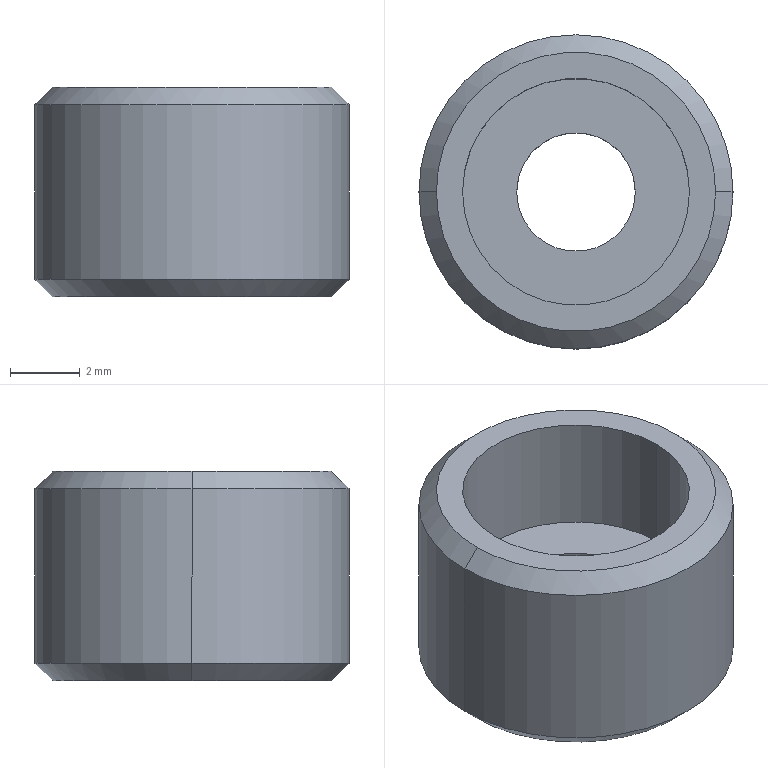Part | STEP file | Anti-rot sleeve | 1 solid | 13 faces | box 9 x 9 x 6 mm | volume 238.468 mm3 | cylinder 6 | cone 4 | plane 3 | commonest cylinder face diameters 3.4 x2 6.5 x2 9 x2
STEP:
#1=CARTESIAN_POINT('',(0.,0.,0.));
#2=DIRECTION('',(0.,0.,1.));
#3=DIRECTION('',(1.,0.,0.));
#4=AXIS2_PLACEMENT_3D('',#1,#2,#3);
#5=CARTESIAN_POINT('',(-4.5,0.,5.5));
#6=VERTEX_POINT('',#5);
#7=CARTESIAN_POINT('',(4.5,0.,5.5));
#8=VERTEX_POINT('',#7);
#9=CARTESIAN_POINT('',(0.,0.,5.5));
#10=DIRECTION('',(0.,0.,-1.));
#11=DIRECTION('',(-1.,0.,0.));
#12=AXIS2_PLACEMENT_3D('',#9,#10,#11);
#13=CIRCLE('',#12,4.5);
#14=CARTESIAN_POINT('',(0.,0.,6.));
#15=DIRECTION('',(0.,0.,-1.));
#16=DIRECTION('',(-1.,0.,0.));
#17=AXIS2_PLACEMENT_3D('',#14,#15,#16);
#18=CYLINDRICAL_SURFACE('',#17,4.5);
#19=CARTESIAN_POINT('',(0.,0.5));
#20=DIRECTION('',(1.,0.));
#21=VECTOR('',#20,1.);
#22=LINE('',#19,#21);
#23=(GEOMETRIC_REPRESENTATION_CONTEXT(2)PARAMETRIC_REPRESENTATION_CONTEXT()REPRESENTATION_CONTEXT('',''));
#24=DEFINITIONAL_REPRESENTATION('',(#22),#23);
#25=PCURVE('',#18,#24);
#26=CARTESIAN_POINT('',(0.,0.,5.5));
#27=DIRECTION('',(0.,0.,-1.));
#28=DIRECTION('',(-1.,0.,0.));
#29=AXIS2_PLACEMENT_3D('',#26,#27,#28);
#30=CONICAL_SURFACE('',#29,4.5,0.7854);
#31=CARTESIAN_POINT('',(0.,0.));
#32=DIRECTION('',(1.,0.));
#33=VECTOR('',#32,1.);
#34=LINE('',#31,#33);
#35=(GEOMETRIC_REPRESENTATION_CONTEXT(2)PARAMETRIC_REPRESENTATION_CONTEXT()REPRESENTATION_CONTEXT('',''));
#36=DEFINITIONAL_REPRESENTATION('',(#34),#35);
#37=PCURVE('',#30,#36);
#38=SURFACE_CURVE('',#13,(#25,#37),.PCURVE_S1.);
#39=EDGE_CURVE('',#6,#8,#38,.T.);
#40=ORIENTED_EDGE('',*,*,#39,.T.);
#41=CARTESIAN_POINT('',(4.5,0.,0.5));
#42=VERTEX_POINT('',#41);
#43=CARTESIAN_POINT('',(4.5,0.,6.));
#44=DIRECTION('',(0.,0.,-1.));
#45=VECTOR('',#44,1.);
#46=LINE('',#43,#45);
#47=CARTESIAN_POINT('',(3.142,0.));
#48=DIRECTION('',(0.,1.));
#49=VECTOR('',#48,1.);
#50=LINE('',#47,#49);
#51=(GEOMETRIC_REPRESENTATION_CONTEXT(2)PARAMETRIC_REPRESENTATION_CONTEXT()REPRESENTATION_CONTEXT('',''));
#52=DEFINITIONAL_REPRESENTATION('',(#50),#51);
#53=PCURVE('',#18,#52);
#54=CARTESIAN_POINT('',(0.,0.,6.));
#55=DIRECTION('',(0.,0.,-1.));
#56=DIRECTION('',(-1.,0.,0.));
#57=AXIS2_PLACEMENT_3D('',#54,#55,#56);
#58=CYLINDRICAL_SURFACE('',#57,4.5);
#59=CARTESIAN_POINT('',(3.142,0.));
#60=DIRECTION('',(0.,1.));
#61=VECTOR('',#60,1.);
#62=LINE('',#59,#61);
#63=(GEOMETRIC_REPRESENTATION_CONTEXT(2)PARAMETRIC_REPRESENTATION_CONTEXT()REPRESENTATION_CONTEXT('',''));
#64=DEFINITIONAL_REPRESENTATION('',(#62),#63);
#65=PCURVE('',#58,#64);
#66=SURFACE_CURVE('',#46,(#53,#65),.PCURVE_S1.);
#67=EDGE_CURVE('',#8,#42,#66,.T.);
#68=ORIENTED_EDGE('',*,*,#67,.T.);
#69=CARTESIAN_POINT('',(-4.5,0.,0.5));
#70=VERTEX_POINT('',#69);
#71=CARTESIAN_POINT('',(0.,0.,0.5));
#72=DIRECTION('',(0.,0.,1.));
#73=DIRECTION('',(-1.,0.,0.));
#74=AXIS2_PLACEMENT_3D('',#71,#72,#73);
#75=CIRCLE('',#74,4.5);
#76=CARTESIAN_POINT('',(6.283,5.5));
#77=DIRECTION('',(-1.,0.));
#78=VECTOR('',#77,1.);
#79=LINE('',#76,#78);
#80=(GEOMETRIC_REPRESENTATION_CONTEXT(2)PARAMETRIC_REPRESENTATION_CONTEXT()REPRESENTATION_CONTEXT('',''));
#81=DEFINITIONAL_REPRESENTATION('',(#79),#80);
#82=PCURVE('',#18,#81);
#83=CARTESIAN_POINT('',(0.,0.,0.5));
#84=DIRECTION('',(0.,0.,1.));
#85=DIRECTION('',(1.,0.,0.));
#86=AXIS2_PLACEMENT_3D('',#83,#84,#85);
#87=CONICAL_SURFACE('',#86,4.5,0.7854);
#88=CARTESIAN_POINT('',(-3.142,0.));
#89=DIRECTION('',(1.,0.));
#90=VECTOR('',#89,1.);
#91=LINE('',#88,#90);
#92=(GEOMETRIC_REPRESENTATION_CONTEXT(2)PARAMETRIC_REPRESENTATION_CONTEXT()REPRESENTATION_CONTEXT('',''));
#93=DEFINITIONAL_REPRESENTATION('',(#91),#92);
#94=PCURVE('',#87,#93);
#95=SURFACE_CURVE('',#75,(#82,#94),.PCURVE_S1.);
#96=EDGE_CURVE('',#42,#70,#95,.T.);
#97=ORIENTED_EDGE('',*,*,#96,.T.);
#98=CARTESIAN_POINT('',(-4.5,0.,6.));
#99=DIRECTION('',(0.,0.,-1.));
#100=VECTOR('',#99,1.);
#101=LINE('',#98,#100);
#102=CARTESIAN_POINT('',(0.,0.));
#103=DIRECTION('',(0.,1.));
#104=VECTOR('',#103,1.);
#105=LINE('',#102,#104);
#106=(GEOMETRIC_REPRESENTATION_CONTEXT(2)PARAMETRIC_REPRESENTATION_CONTEXT()REPRESENTATION_CONTEXT('',''));
#107=DEFINITIONAL_REPRESENTATION('',(#105),#106);
#108=PCURVE('',#18,#107);
#109=CARTESIAN_POINT('',(6.283,0.));
#110=DIRECTION('',(0.,1.));
#111=VECTOR('',#110,1.);
#112=LINE('',#109,#111);
#113=(GEOMETRIC_REPRESENTATION_CONTEXT(2)PARAMETRIC_REPRESENTATION_CONTEXT()REPRESENTATION_CONTEXT('',''));
#114=DEFINITIONAL_REPRESENTATION('',(#112),#113);
#115=PCURVE('',#58,#114);
#116=SURFACE_CURVE('',#101,(#108,#115),.PCURVE_S1.);
#117=EDGE_CURVE('',#6,#70,#116,.T.);
#118=ORIENTED_EDGE('',*,*,#117,.F.);
#119=EDGE_LOOP('',(#40,#68,#97,#118));
#120=FACE_BOUND('',#119,.T.);
#121=ADVANCED_FACE('',(#120),#18,.T.);
#122=CARTESIAN_POINT('',(4.,0.,0.));
#123=VERTEX_POINT('',#122);
#124=CARTESIAN_POINT('',(-4.,0.,0.));
#125=VERTEX_POINT('',#124);
#126=CARTESIAN_POINT('',(0.,0.,0.));
#127=DIRECTION('',(0.,0.,1.));
#128=DIRECTION('',(1.,0.,0.));
#129=AXIS2_PLACEMENT_3D('',#126,#127,#128);
#130=CIRCLE('',#129,4.);
#131=CARTESIAN_POINT('',(0.,-0.5));
#132=DIRECTION('',(1.,0.));
#133=VECTOR('',#132,1.);
#134=LINE('',#131,#133);
#135=(GEOMETRIC_REPRESENTATION_CONTEXT(2)PARAMETRIC_REPRESENTATION_CONTEXT()REPRESENTATION_CONTEXT('',''));
#136=DEFINITIONAL_REPRESENTATION('',(#134),#135);
#137=PCURVE('',#87,#136);
#138=CARTESIAN_POINT('',(0.,0.,0.));
#139=DIRECTION('',(0.,0.,1.));
#140=DIRECTION('',(1.,0.,0.));
#141=AXIS2_PLACEMENT_3D('',#138,#139,#140);
#142=PLANE('',#141);
#143=CARTESIAN_POINT('',(0.,0.));
#144=DIRECTION('',(1.,0.));
#145=AXIS2_PLACEMENT_2D('',#143,#144);
#146=CIRCLE('',#145,4.);
#147=(GEOMETRIC_REPRESENTATION_CONTEXT(2)PARAMETRIC_REPRESENTATION_CONTEXT()REPRESENTATION_CONTEXT('',''));
#148=DEFINITIONAL_REPRESENTATION('',(#146),#147);
#149=PCURVE('',#142,#148);
#150=SURFACE_CURVE('',#130,(#137,#149),.PCURVE_S1.);
#151=EDGE_CURVE('',#123,#125,#150,.T.);
#152=ORIENTED_EDGE('',*,*,#151,.T.);
#153=CARTESIAN_POINT('',(-4.5,0.,0.5));
#154=DIRECTION('',(-0.7071,0.,0.7071));
#155=VECTOR('',#154,1.);
#156=LINE('',#153,#155);
#157=CARTESIAN_POINT('',(3.142,0.));
#158=DIRECTION('',(0.,1.));
#159=VECTOR('',#158,1.);
#160=LINE('',#157,#159);
#161=(GEOMETRIC_REPRESENTATION_CONTEXT(2)PARAMETRIC_REPRESENTATION_CONTEXT()REPRESENTATION_CONTEXT('',''));
#162=DEFINITIONAL_REPRESENTATION('',(#160),#161);
#163=PCURVE('',#87,#162);
#164=CARTESIAN_POINT('',(0.,0.,0.5));
#165=DIRECTION('',(0.,0.,1.));
#166=DIRECTION('',(1.,0.,0.));
#167=AXIS2_PLACEMENT_3D('',#164,#165,#166);
#168=CONICAL_SURFACE('',#167,4.5,0.7854);
#169=CARTESIAN_POINT('',(3.142,0.));
#170=DIRECTION('',(0.,1.));
#171=VECTOR('',#170,1.);
#172=LINE('',#169,#171);
#173=(GEOMETRIC_REPRESENTATION_CONTEXT(2)PARAMETRIC_REPRESENTATION_CONTEXT()REPRESENTATION_CONTEXT('',''));
#174=DEFINITIONAL_REPRESENTATION('',(#172),#173);
#175=PCURVE('',#168,#174);
#176=SURFACE_CURVE('',#156,(#163,#175),.PCURVE_S1.);
#177=EDGE_CURVE('',#125,#70,#176,.T.);
#178=ORIENTED_EDGE('',*,*,#177,.T.);
#179=ORIENTED_EDGE('',*,*,#96,.F.);
#180=CARTESIAN_POINT('',(4.5,0.,0.5));
#181=DIRECTION('',(0.7071,0.,0.7071));
#182=VECTOR('',#181,1.);
#183=LINE('',#180,#182);
#184=CARTESIAN_POINT('',(0.,0.));
#185=DIRECTION('',(0.,1.));
#186=VECTOR('',#185,1.);
#187=LINE('',#184,#186);
#188=(GEOMETRIC_REPRESENTATION_CONTEXT(2)PARAMETRIC_REPRESENTATION_CONTEXT()REPRESENTATION_CONTEXT('',''));
#189=DEFINITIONAL_REPRESENTATION('',(#187),#188);
#190=PCURVE('',#87,#189);
#191=CARTESIAN_POINT('',(6.283,0.));
#192=DIRECTION('',(0.,1.));
#193=VECTOR('',#192,1.);
#194=LINE('',#191,#193);
#195=(GEOMETRIC_REPRESENTATION_CONTEXT(2)PARAMETRIC_REPRESENTATION_CONTEXT()REPRESENTATION_CONTEXT('',''));
#196=DEFINITIONAL_REPRESENTATION('',(#194),#195);
#197=PCURVE('',#168,#196);
#198=SURFACE_CURVE('',#183,(#190,#197),.PCURVE_S1.);
#199=EDGE_CURVE('',#123,#42,#198,.T.);
#200=ORIENTED_EDGE('',*,*,#199,.F.);
#201=EDGE_LOOP('',(#152,#178,#179,#200));
#202=FACE_BOUND('',#201,.T.);
#203=ADVANCED_FACE('',(#202),#87,.T.);
#204=CARTESIAN_POINT('',(-4.,0.,6.));
#205=VERTEX_POINT('',#204);
#206=CARTESIAN_POINT('',(4.,0.,6.));
#207=VERTEX_POINT('',#206);
#208=CARTESIAN_POINT('',(0.,0.,6.));
#209=DIRECTION('',(0.,0.,-1.));
#210=DIRECTION('',(-1.,0.,0.));
#211=AXIS2_PLACEMENT_3D('',#208,#209,#210);
#212=CIRCLE('',#211,4.);
#213=CARTESIAN_POINT('',(0.,-0.5));
#214=DIRECTION('',(1.,0.));
#215=VECTOR('',#214,1.);
#216=LINE('',#213,#215);
#217=(GEOMETRIC_REPRESENTATION_CONTEXT(2)PARAMETRIC_REPRESENTATION_CONTEXT()REPRESENTATION_CONTEXT('',''));
#218=DEFINITIONAL_REPRESENTATION('',(#216),#217);
#219=PCURVE('',#30,#218);
#220=CARTESIAN_POINT('',(0.,0.,6.));
#221=DIRECTION('',(0.,0.,1.));
#222=DIRECTION('',(1.,0.,0.));
#223=AXIS2_PLACEMENT_3D('',#220,#221,#222);
#224=PLANE('',#223);
#225=CARTESIAN_POINT('',(-4.,0.));
#226=CARTESIAN_POINT('',(-4.,6.928));
#227=CARTESIAN_POINT('',(2.,3.464));
#228=CARTESIAN_POINT('',(8.,0.));
#229=CARTESIAN_POINT('',(2.,-3.464));
#230=CARTESIAN_POINT('',(-4.,-6.928));
#231=CARTESIAN_POINT('',(-4.,0.));
#232=(BOUNDED_CURVE()B_SPLINE_CURVE(2,(#225,#226,#227,#228,#229,#230,#231),.UNSPECIFIED.,.T.,.F.)B_SPLINE_CURVE_WITH_KNOTS((1,2,2,2,2,1),(-2.094,0.,2.094,4.189,6.283,8.378),.UNSPECIFIED.)CURVE()GEOMETRIC_REPRESENTATION_ITEM()RATIONAL_B_SPLINE_CURVE((1.,0.5,1.,0.5,1.,0.5,1.))REPRESENTATION_ITEM(''));
#233=(GEOMETRIC_REPRESENTATION_CONTEXT(2)PARAMETRIC_REPRESENTATION_CONTEXT()REPRESENTATION_CONTEXT('',''));
#234=DEFINITIONAL_REPRESENTATION('',(#232),#233);
#235=PCURVE('',#224,#234);
#236=SURFACE_CURVE('',#212,(#219,#235),.PCURVE_S1.);
#237=EDGE_CURVE('',#205,#207,#236,.T.);
#238=ORIENTED_EDGE('',*,*,#237,.T.);
#239=CARTESIAN_POINT('',(4.5,0.,5.5));
#240=DIRECTION('',(0.7071,0.,-0.7071));
#241=VECTOR('',#240,1.);
#242=LINE('',#239,#241);
#243=CARTESIAN_POINT('',(3.142,0.));
#244=DIRECTION('',(0.,1.));
#245=VECTOR('',#244,1.);
#246=LINE('',#243,#245);
#247=(GEOMETRIC_REPRESENTATION_CONTEXT(2)PARAMETRIC_REPRESENTATION_CONTEXT()REPRESENTATION_CONTEXT('',''));
#248=DEFINITIONAL_REPRESENTATION('',(#246),#247);
#249=PCURVE('',#30,#248);
#250=CARTESIAN_POINT('',(0.,0.,5.5));
#251=DIRECTION('',(0.,0.,-1.));
#252=DIRECTION('',(-1.,0.,0.));
#253=AXIS2_PLACEMENT_3D('',#250,#251,#252);
#254=CONICAL_SURFACE('',#253,4.5,0.7854);
#255=CARTESIAN_POINT('',(3.142,0.));
#256=DIRECTION('',(0.,1.));
#257=VECTOR('',#256,1.);
#258=LINE('',#255,#257);
#259=(GEOMETRIC_REPRESENTATION_CONTEXT(2)PARAMETRIC_REPRESENTATION_CONTEXT()REPRESENTATION_CONTEXT('',''));
#260=DEFINITIONAL_REPRESENTATION('',(#258),#259);
#261=PCURVE('',#254,#260);
#262=SURFACE_CURVE('',#242,(#249,#261),.PCURVE_S1.);
#263=EDGE_CURVE('',#207,#8,#262,.T.);
#264=ORIENTED_EDGE('',*,*,#263,.T.);
#265=ORIENTED_EDGE('',*,*,#39,.F.);
#266=CARTESIAN_POINT('',(-4.5,0.,5.5));
#267=DIRECTION('',(-0.7071,0.,-0.7071));
#268=VECTOR('',#267,1.);
#269=LINE('',#266,#268);
#270=CARTESIAN_POINT('',(0.,0.));
#271=DIRECTION('',(0.,1.));
#272=VECTOR('',#271,1.);
#273=LINE('',#270,#272);
#274=(GEOMETRIC_REPRESENTATION_CONTEXT(2)PARAMETRIC_REPRESENTATION_CONTEXT()REPRESENTATION_CONTEXT('',''));
#275=DEFINITIONAL_REPRESENTATION('',(#273),#274);
#276=PCURVE('',#30,#275);
#277=CARTESIAN_POINT('',(6.283,0.));
#278=DIRECTION('',(0.,1.));
#279=VECTOR('',#278,1.);
#280=LINE('',#277,#279);
#281=(GEOMETRIC_REPRESENTATION_CONTEXT(2)PARAMETRIC_REPRESENTATION_CONTEXT()REPRESENTATION_CONTEXT('',''));
#282=DEFINITIONAL_REPRESENTATION('',(#280),#281);
#283=PCURVE('',#254,#282);
#284=SURFACE_CURVE('',#269,(#276,#283),.PCURVE_S1.);
#285=EDGE_CURVE('',#205,#6,#284,.T.);
#286=ORIENTED_EDGE('',*,*,#285,.F.);
#287=EDGE_LOOP('',(#238,#264,#265,#286));
#288=FACE_BOUND('',#287,.T.);
#289=ADVANCED_FACE('',(#288),#30,.T.);
#290=CARTESIAN_POINT('',(1.7,0.,0.));
#291=VERTEX_POINT('',#290);
#292=CARTESIAN_POINT('',(1.7,0.,2.6));
#293=VERTEX_POINT('',#292);
#294=CARTESIAN_POINT('',(1.7,0.,6.));
#295=DIRECTION('',(0.,0.,1.));
#296=VECTOR('',#295,1.);
#297=LINE('',#294,#296);
#298=CARTESIAN_POINT('',(0.,0.,6.));
#299=DIRECTION('',(0.,0.,1.));
#300=DIRECTION('',(1.,0.,0.));
#301=AXIS2_PLACEMENT_3D('',#298,#299,#300);
#302=CYLINDRICAL_SURFACE('',#301,1.7);
#303=CARTESIAN_POINT('',(6.283,0.));
#304=DIRECTION('',(0.,1.));
#305=VECTOR('',#304,1.);
#306=LINE('',#303,#305);
#307=(GEOMETRIC_REPRESENTATION_CONTEXT(2)PARAMETRIC_REPRESENTATION_CONTEXT()REPRESENTATION_CONTEXT('',''));
#308=DEFINITIONAL_REPRESENTATION('',(#306),#307);
#309=PCURVE('',#302,#308);
#310=CARTESIAN_POINT('',(0.,0.,6.));
#311=DIRECTION('',(0.,0.,1.));
#312=DIRECTION('',(1.,0.,0.));
#313=AXIS2_PLACEMENT_3D('',#310,#311,#312);
#314=CYLINDRICAL_SURFACE('',#313,1.7);
#315=CARTESIAN_POINT('',(0.,0.));
#316=DIRECTION('',(0.,1.));
#317=VECTOR('',#316,1.);
#318=LINE('',#315,#317);
#319=(GEOMETRIC_REPRESENTATION_CONTEXT(2)PARAMETRIC_REPRESENTATION_CONTEXT()REPRESENTATION_CONTEXT('',''));
#320=DEFINITIONAL_REPRESENTATION('',(#318),#319);
#321=PCURVE('',#314,#320);
#322=SURFACE_CURVE('',#297,(#309,#321),.PCURVE_S1.);
#323=EDGE_CURVE('',#291,#293,#322,.T.);
#324=ORIENTED_EDGE('',*,*,#323,.T.);
#325=CARTESIAN_POINT('',(-1.7,0.,2.6));
#326=VERTEX_POINT('',#325);
#327=CARTESIAN_POINT('',(0.,0.,2.6));
#328=DIRECTION('',(0.,0.,-1.));
#329=DIRECTION('',(1.,0.,0.));
#330=AXIS2_PLACEMENT_3D('',#327,#328,#329);
#331=CIRCLE('',#330,1.7);
#332=CARTESIAN_POINT('',(6.283,-3.4));
#333=DIRECTION('',(-1.,0.));
#334=VECTOR('',#333,1.);
#335=LINE('',#332,#334);
#336=(GEOMETRIC_REPRESENTATION_CONTEXT(2)PARAMETRIC_REPRESENTATION_CONTEXT()REPRESENTATION_CONTEXT('',''));
#337=DEFINITIONAL_REPRESENTATION('',(#335),#336);
#338=PCURVE('',#302,#337);
#339=CARTESIAN_POINT('',(1.7,0.,2.6));
#340=DIRECTION('',(0.,0.,-1.));
#341=DIRECTION('',(-1.,0.,0.));
#342=AXIS2_PLACEMENT_3D('',#339,#340,#341);
#343=PLANE('',#342);
#344=CARTESIAN_POINT('',(1.7,0.));
#345=DIRECTION('',(-1.,0.));
#346=AXIS2_PLACEMENT_2D('',#344,#345);
#347=CIRCLE('',#346,1.7);
#348=(GEOMETRIC_REPRESENTATION_CONTEXT(2)PARAMETRIC_REPRESENTATION_CONTEXT()REPRESENTATION_CONTEXT('',''));
#349=DEFINITIONAL_REPRESENTATION('',(#347),#348);
#350=PCURVE('',#343,#349);
#351=SURFACE_CURVE('',#331,(#338,#350),.PCURVE_S1.);
#352=EDGE_CURVE('',#293,#326,#351,.T.);
#353=ORIENTED_EDGE('',*,*,#352,.T.);
#354=CARTESIAN_POINT('',(-1.7,0.,0.));
#355=VERTEX_POINT('',#354);
#356=CARTESIAN_POINT('',(-1.7,0.,6.));
#357=DIRECTION('',(0.,0.,1.));
#358=VECTOR('',#357,1.);
#359=LINE('',#356,#358);
#360=CARTESIAN_POINT('',(3.142,0.));
#361=DIRECTION('',(0.,1.));
#362=VECTOR('',#361,1.);
#363=LINE('',#360,#362);
#364=(GEOMETRIC_REPRESENTATION_CONTEXT(2)PARAMETRIC_REPRESENTATION_CONTEXT()REPRESENTATION_CONTEXT('',''));
#365=DEFINITIONAL_REPRESENTATION('',(#363),#364);
#366=PCURVE('',#302,#365);
#367=CARTESIAN_POINT('',(3.142,0.));
#368=DIRECTION('',(0.,1.));
#369=VECTOR('',#368,1.);
#370=LINE('',#367,#369);
#371=(GEOMETRIC_REPRESENTATION_CONTEXT(2)PARAMETRIC_REPRESENTATION_CONTEXT()REPRESENTATION_CONTEXT('',''));
#372=DEFINITIONAL_REPRESENTATION('',(#370),#371);
#373=PCURVE('',#314,#372);
#374=SURFACE_CURVE('',#359,(#366,#373),.PCURVE_S1.);
#375=EDGE_CURVE('',#355,#326,#374,.T.);
#376=ORIENTED_EDGE('',*,*,#375,.F.);
#377=CARTESIAN_POINT('',(0.,0.,0.));
#378=DIRECTION('',(0.,0.,-1.));
#379=DIRECTION('',(1.,0.,0.));
#380=AXIS2_PLACEMENT_3D('',#377,#378,#379);
#381=CIRCLE('',#380,1.7);
#382=CARTESIAN_POINT('',(6.283,-6.));
#383=DIRECTION('',(-1.,0.));
#384=VECTOR('',#383,1.);
#385=LINE('',#382,#384);
#386=(GEOMETRIC_REPRESENTATION_CONTEXT(2)PARAMETRIC_REPRESENTATION_CONTEXT()REPRESENTATION_CONTEXT('',''));
#387=DEFINITIONAL_REPRESENTATION('',(#385),#386);
#388=PCURVE('',#302,#387);
#389=CARTESIAN_POINT('',(1.7,0.));
#390=CARTESIAN_POINT('',(1.7,-2.944));
#391=CARTESIAN_POINT('',(-0.85,-1.472));
#392=CARTESIAN_POINT('',(-3.4,0.));
#393=CARTESIAN_POINT('',(-0.85,1.472));
#394=CARTESIAN_POINT('',(1.7,2.944));
#395=CARTESIAN_POINT('',(1.7,0.));
#396=(BOUNDED_CURVE()B_SPLINE_CURVE(2,(#389,#390,#391,#392,#393,#394,#395),.UNSPECIFIED.,.T.,.F.)B_SPLINE_CURVE_WITH_KNOTS((1,2,2,2,2,1),(-2.094,0.,2.094,4.189,6.283,8.378),.UNSPECIFIED.)CURVE()GEOMETRIC_REPRESENTATION_ITEM()RATIONAL_B_SPLINE_CURVE((1.,0.5,1.,0.5,1.,0.5,1.))REPRESENTATION_ITEM(''));
#397=(GEOMETRIC_REPRESENTATION_CONTEXT(2)PARAMETRIC_REPRESENTATION_CONTEXT()REPRESENTATION_CONTEXT('',''));
#398=DEFINITIONAL_REPRESENTATION('',(#396),#397);
#399=PCURVE('',#142,#398);
#400=SURFACE_CURVE('',#381,(#388,#399),.PCURVE_S1.);
#401=EDGE_CURVE('',#291,#355,#400,.T.);
#402=ORIENTED_EDGE('',*,*,#401,.F.);
#403=EDGE_LOOP('',(#324,#353,#376,#402));
#404=FACE_BOUND('',#403,.F.);
#405=ADVANCED_FACE('',(#404),#302,.F.);
#406=CARTESIAN_POINT('',(3.25,0.,2.6));
#407=VERTEX_POINT('',#406);
#408=CARTESIAN_POINT('',(3.25,0.,6.));
#409=VERTEX_POINT('',#408);
#410=CARTESIAN_POINT('',(3.25,0.,6.));
#411=DIRECTION('',(0.,0.,1.));
#412=VECTOR('',#411,1.);
#413=LINE('',#410,#412);
#414=CARTESIAN_POINT('',(0.,0.,6.));
#415=DIRECTION('',(0.,0.,1.));
#416=DIRECTION('',(1.,0.,0.));
#417=AXIS2_PLACEMENT_3D('',#414,#415,#416);
#418=CYLINDRICAL_SURFACE('',#417,3.25);
#419=CARTESIAN_POINT('',(6.283,0.));
#420=DIRECTION('',(0.,1.));
#421=VECTOR('',#420,1.);
#422=LINE('',#419,#421);
#423=(GEOMETRIC_REPRESENTATION_CONTEXT(2)PARAMETRIC_REPRESENTATION_CONTEXT()REPRESENTATION_CONTEXT('',''));
#424=DEFINITIONAL_REPRESENTATION('',(#422),#423);
#425=PCURVE('',#418,#424);
#426=CARTESIAN_POINT('',(0.,0.,6.));
#427=DIRECTION('',(0.,0.,1.));
#428=DIRECTION('',(1.,0.,0.));
#429=AXIS2_PLACEMENT_3D('',#426,#427,#428);
#430=CYLINDRICAL_SURFACE('',#429,3.25);
#431=CARTESIAN_POINT('',(0.,0.));
#432=DIRECTION('',(0.,1.));
#433=VECTOR('',#432,1.);
#434=LINE('',#431,#433);
#435=(GEOMETRIC_REPRESENTATION_CONTEXT(2)PARAMETRIC_REPRESENTATION_CONTEXT()REPRESENTATION_CONTEXT('',''));
#436=DEFINITIONAL_REPRESENTATION('',(#434),#435);
#437=PCURVE('',#430,#436);
#438=SURFACE_CURVE('',#413,(#425,#437),.PCURVE_S1.);
#439=EDGE_CURVE('',#407,#409,#438,.T.);
#440=ORIENTED_EDGE('',*,*,#439,.T.);
#441=CARTESIAN_POINT('',(-3.25,0.,6.));
#442=VERTEX_POINT('',#441);
#443=CARTESIAN_POINT('',(0.,0.,6.));
#444=DIRECTION('',(0.,0.,-1.));
#445=DIRECTION('',(1.,0.,0.));
#446=AXIS2_PLACEMENT_3D('',#443,#444,#445);
#447=CIRCLE('',#446,3.25);
#448=CARTESIAN_POINT('',(6.283,0.));
#449=DIRECTION('',(-1.,0.));
#450=VECTOR('',#449,1.);
#451=LINE('',#448,#450);
#452=(GEOMETRIC_REPRESENTATION_CONTEXT(2)PARAMETRIC_REPRESENTATION_CONTEXT()REPRESENTATION_CONTEXT('',''));
#453=DEFINITIONAL_REPRESENTATION('',(#451),#452);
#454=PCURVE('',#418,#453);
#455=CARTESIAN_POINT('',(3.25,0.));
#456=CARTESIAN_POINT('',(3.25,-5.629));
#457=CARTESIAN_POINT('',(-1.625,-2.815));
#458=CARTESIAN_POINT('',(-6.5,0.));
#459=CARTESIAN_POINT('',(-1.625,2.815));
#460=CARTESIAN_POINT('',(3.25,5.629));
#461=CARTESIAN_POINT('',(3.25,0.));
#462=(BOUNDED_CURVE()B_SPLINE_CURVE(2,(#455,#456,#457,#458,#459,#460,#461),.UNSPECIFIED.,.T.,.F.)B_SPLINE_CURVE_WITH_KNOTS((1,2,2,2,2,1),(-2.094,0.,2.094,4.189,6.283,8.378),.UNSPECIFIED.)CURVE()GEOMETRIC_REPRESENTATION_ITEM()RATIONAL_B_SPLINE_CURVE((1.,0.5,1.,0.5,1.,0.5,1.))REPRESENTATION_ITEM(''));
#463=(GEOMETRIC_REPRESENTATION_CONTEXT(2)PARAMETRIC_REPRESENTATION_CONTEXT()REPRESENTATION_CONTEXT('',''));
#464=DEFINITIONAL_REPRESENTATION('',(#462),#463);
#465=PCURVE('',#224,#464);
#466=SURFACE_CURVE('',#447,(#454,#465),.PCURVE_S1.);
#467=EDGE_CURVE('',#409,#442,#466,.T.);
#468=ORIENTED_EDGE('',*,*,#467,.T.);
#469=CARTESIAN_POINT('',(-3.25,0.,2.6));
#470=VERTEX_POINT('',#469);
#471=CARTESIAN_POINT('',(-3.25,0.,6.));
#472=DIRECTION('',(0.,0.,1.));
#473=VECTOR('',#472,1.);
#474=LINE('',#471,#473);
#475=CARTESIAN_POINT('',(3.142,0.));
#476=DIRECTION('',(0.,1.));
#477=VECTOR('',#476,1.);
#478=LINE('',#475,#477);
#479=(GEOMETRIC_REPRESENTATION_CONTEXT(2)PARAMETRIC_REPRESENTATION_CONTEXT()REPRESENTATION_CONTEXT('',''));
#480=DEFINITIONAL_REPRESENTATION('',(#478),#479);
#481=PCURVE('',#418,#480);
#482=CARTESIAN_POINT('',(3.142,0.));
#483=DIRECTION('',(0.,1.));
#484=VECTOR('',#483,1.);
#485=LINE('',#482,#484);
#486=(GEOMETRIC_REPRESENTATION_CONTEXT(2)PARAMETRIC_REPRESENTATION_CONTEXT()REPRESENTATION_CONTEXT('',''));
#487=DEFINITIONAL_REPRESENTATION('',(#485),#486);
#488=PCURVE('',#430,#487);
#489=SURFACE_CURVE('',#474,(#481,#488),.PCURVE_S1.);
#490=EDGE_CURVE('',#470,#442,#489,.T.);
#491=ORIENTED_EDGE('',*,*,#490,.F.);
#492=CARTESIAN_POINT('',(0.,0.,2.6));
#493=DIRECTION('',(0.,0.,1.));
#494=DIRECTION('',(1.,0.,0.));
#495=AXIS2_PLACEMENT_3D('',#492,#493,#494);
#496=CIRCLE('',#495,3.25);
#497=CARTESIAN_POINT('',(0.,-3.4));
#498=DIRECTION('',(1.,0.));
#499=VECTOR('',#498,1.);
#500=LINE('',#497,#499);
#501=(GEOMETRIC_REPRESENTATION_CONTEXT(2)PARAMETRIC_REPRESENTATION_CONTEXT()REPRESENTATION_CONTEXT('',''));
#502=DEFINITIONAL_REPRESENTATION('',(#500),#501);
#503=PCURVE('',#418,#502);
#504=CARTESIAN_POINT('',(-1.55,0.));
#505=CARTESIAN_POINT('',(-1.55,5.629));
#506=CARTESIAN_POINT('',(3.325,2.815));
#507=CARTESIAN_POINT('',(8.2,0.));
#508=CARTESIAN_POINT('',(3.325,-2.815));
#509=CARTESIAN_POINT('',(-1.55,-5.629));
#510=CARTESIAN_POINT('',(-1.55,0.));
#511=(BOUNDED_CURVE()B_SPLINE_CURVE(2,(#504,#505,#506,#507,#508,#509,#510),.UNSPECIFIED.,.T.,.F.)B_SPLINE_CURVE_WITH_KNOTS((1,2,2,2,2,1),(-2.094,0.,2.094,4.189,6.283,8.378),.UNSPECIFIED.)CURVE()GEOMETRIC_REPRESENTATION_ITEM()RATIONAL_B_SPLINE_CURVE((1.,0.5,1.,0.5,1.,0.5,1.))REPRESENTATION_ITEM(''));
#512=(GEOMETRIC_REPRESENTATION_CONTEXT(2)PARAMETRIC_REPRESENTATION_CONTEXT()REPRESENTATION_CONTEXT('',''));
#513=DEFINITIONAL_REPRESENTATION('',(#511),#512);
#514=PCURVE('',#343,#513);
#515=SURFACE_CURVE('',#496,(#503,#514),.PCURVE_S1.);
#516=EDGE_CURVE('',#470,#407,#515,.T.);
#517=ORIENTED_EDGE('',*,*,#516,.T.);
#518=EDGE_LOOP('',(#440,#468,#491,#517));
#519=FACE_BOUND('',#518,.F.);
#520=ADVANCED_FACE('',(#519),#418,.F.);
#521=ORIENTED_EDGE('',*,*,#67,.F.);
#522=CARTESIAN_POINT('',(0.,0.,5.5));
#523=DIRECTION('',(0.,0.,-1.));
#524=DIRECTION('',(-1.,0.,0.));
#525=AXIS2_PLACEMENT_3D('',#522,#523,#524);
#526=CIRCLE('',#525,4.5);
#527=CARTESIAN_POINT('',(0.,0.5));
#528=DIRECTION('',(1.,0.));
#529=VECTOR('',#528,1.);
#530=LINE('',#527,#529);
#531=(GEOMETRIC_REPRESENTATION_CONTEXT(2)PARAMETRIC_REPRESENTATION_CONTEXT()REPRESENTATION_CONTEXT('',''));
#532=DEFINITIONAL_REPRESENTATION('',(#530),#531);
#533=PCURVE('',#58,#532);
#534=CARTESIAN_POINT('',(0.,0.));
#535=DIRECTION('',(1.,0.));
#536=VECTOR('',#535,1.);
#537=LINE('',#534,#536);
#538=(GEOMETRIC_REPRESENTATION_CONTEXT(2)PARAMETRIC_REPRESENTATION_CONTEXT()REPRESENTATION_CONTEXT('',''));
#539=DEFINITIONAL_REPRESENTATION('',(#537),#538);
#540=PCURVE('',#254,#539);
#541=SURFACE_CURVE('',#526,(#533,#540),.PCURVE_S1.);
#542=EDGE_CURVE('',#8,#6,#541,.T.);
#543=ORIENTED_EDGE('',*,*,#542,.T.);
#544=ORIENTED_EDGE('',*,*,#117,.T.);
#545=CARTESIAN_POINT('',(0.,0.,0.5));
#546=DIRECTION('',(0.,0.,1.));
#547=DIRECTION('',(-1.,0.,0.));
#548=AXIS2_PLACEMENT_3D('',#545,#546,#547);
#549=CIRCLE('',#548,4.5);
#550=CARTESIAN_POINT('',(6.283,5.5));
#551=DIRECTION('',(-1.,0.));
#552=VECTOR('',#551,1.);
#553=LINE('',#550,#552);
#554=(GEOMETRIC_REPRESENTATION_CONTEXT(2)PARAMETRIC_REPRESENTATION_CONTEXT()REPRESENTATION_CONTEXT('',''));
#555=DEFINITIONAL_REPRESENTATION('',(#553),#554);
#556=PCURVE('',#58,#555);
#557=CARTESIAN_POINT('',(3.142,0.));
#558=DIRECTION('',(1.,0.));
#559=VECTOR('',#558,1.);
#560=LINE('',#557,#559);
#561=(GEOMETRIC_REPRESENTATION_CONTEXT(2)PARAMETRIC_REPRESENTATION_CONTEXT()REPRESENTATION_CONTEXT('',''));
#562=DEFINITIONAL_REPRESENTATION('',(#560),#561);
#563=PCURVE('',#168,#562);
#564=SURFACE_CURVE('',#549,(#556,#563),.PCURVE_S1.);
#565=EDGE_CURVE('',#70,#42,#564,.T.);
#566=ORIENTED_EDGE('',*,*,#565,.T.);
#567=EDGE_LOOP('',(#521,#543,#544,#566));
#568=FACE_BOUND('',#567,.T.);
#569=ADVANCED_FACE('',(#568),#58,.T.);
#570=ORIENTED_EDGE('',*,*,#177,.F.);
#571=CARTESIAN_POINT('',(0.,0.,0.));
#572=DIRECTION('',(0.,0.,1.));
#573=DIRECTION('',(1.,0.,0.));
#574=AXIS2_PLACEMENT_3D('',#571,#572,#573);
#575=CIRCLE('',#574,4.);
#576=CARTESIAN_POINT('',(0.,-0.5));
#577=DIRECTION('',(1.,0.));
#578=VECTOR('',#577,1.);
#579=LINE('',#576,#578);
#580=(GEOMETRIC_REPRESENTATION_CONTEXT(2)PARAMETRIC_REPRESENTATION_CONTEXT()REPRESENTATION_CONTEXT('',''));
#581=DEFINITIONAL_REPRESENTATION('',(#579),#580);
#582=PCURVE('',#168,#581);
#583=CARTESIAN_POINT('',(0.,0.));
#584=DIRECTION('',(1.,0.));
#585=AXIS2_PLACEMENT_2D('',#583,#584);
#586=CIRCLE('',#585,4.);
#587=(GEOMETRIC_REPRESENTATION_CONTEXT(2)PARAMETRIC_REPRESENTATION_CONTEXT()REPRESENTATION_CONTEXT('',''));
#588=DEFINITIONAL_REPRESENTATION('',(#586),#587);
#589=PCURVE('',#142,#588);
#590=SURFACE_CURVE('',#575,(#582,#589),.PCURVE_S1.);
#591=EDGE_CURVE('',#125,#123,#590,.T.);
#592=ORIENTED_EDGE('',*,*,#591,.T.);
#593=ORIENTED_EDGE('',*,*,#199,.T.);
#594=ORIENTED_EDGE('',*,*,#565,.F.);
#595=EDGE_LOOP('',(#570,#592,#593,#594));
#596=FACE_BOUND('',#595,.T.);
#597=ADVANCED_FACE('',(#596),#168,.T.);
#598=ORIENTED_EDGE('',*,*,#263,.F.);
#599=CARTESIAN_POINT('',(0.,0.,6.));
#600=DIRECTION('',(0.,0.,-1.));
#601=DIRECTION('',(-1.,0.,0.));
#602=AXIS2_PLACEMENT_3D('',#599,#600,#601);
#603=CIRCLE('',#602,4.);
#604=CARTESIAN_POINT('',(0.,-0.5));
#605=DIRECTION('',(1.,0.));
#606=VECTOR('',#605,1.);
#607=LINE('',#604,#606);
#608=(GEOMETRIC_REPRESENTATION_CONTEXT(2)PARAMETRIC_REPRESENTATION_CONTEXT()REPRESENTATION_CONTEXT('',''));
#609=DEFINITIONAL_REPRESENTATION('',(#607),#608);
#610=PCURVE('',#254,#609);
#611=CARTESIAN_POINT('',(-4.,0.));
#612=CARTESIAN_POINT('',(-4.,6.928));
#613=CARTESIAN_POINT('',(2.,3.464));
#614=CARTESIAN_POINT('',(8.,0.));
#615=CARTESIAN_POINT('',(2.,-3.464));
#616=CARTESIAN_POINT('',(-4.,-6.928));
#617=CARTESIAN_POINT('',(-4.,0.));
#618=(BOUNDED_CURVE()B_SPLINE_CURVE(2,(#611,#612,#613,#614,#615,#616,#617),.UNSPECIFIED.,.T.,.F.)B_SPLINE_CURVE_WITH_KNOTS((1,2,2,2,2,1),(-2.094,0.,2.094,4.189,6.283,8.378),.UNSPECIFIED.)CURVE()GEOMETRIC_REPRESENTATION_ITEM()RATIONAL_B_SPLINE_CURVE((1.,0.5,1.,0.5,1.,0.5,1.))REPRESENTATION_ITEM(''));
#619=(GEOMETRIC_REPRESENTATION_CONTEXT(2)PARAMETRIC_REPRESENTATION_CONTEXT()REPRESENTATION_CONTEXT('',''));
#620=DEFINITIONAL_REPRESENTATION('',(#618),#619);
#621=PCURVE('',#224,#620);
#622=SURFACE_CURVE('',#603,(#610,#621),.PCURVE_S1.);
#623=EDGE_CURVE('',#207,#205,#622,.T.);
#624=ORIENTED_EDGE('',*,*,#623,.T.);
#625=ORIENTED_EDGE('',*,*,#285,.T.);
#626=ORIENTED_EDGE('',*,*,#542,.F.);
#627=EDGE_LOOP('',(#598,#624,#625,#626));
#628=FACE_BOUND('',#627,.T.);
#629=ADVANCED_FACE('',(#628),#254,.T.);
#630=ORIENTED_EDGE('',*,*,#401,.F.);
#631=CARTESIAN_POINT('',(0.,0.,0.));
#632=DIRECTION('',(0.,0.,-1.));
#633=DIRECTION('',(1.,0.,0.));
#634=AXIS2_PLACEMENT_3D('',#631,#632,#633);
#635=CIRCLE('',#634,1.7);
#636=CARTESIAN_POINT('',(1.7,0.));
#637=CARTESIAN_POINT('',(1.7,-2.944));
#638=CARTESIAN_POINT('',(-0.85,-1.472));
#639=CARTESIAN_POINT('',(-3.4,0.));
#640=CARTESIAN_POINT('',(-0.85,1.472));
#641=CARTESIAN_POINT('',(1.7,2.944));
#642=CARTESIAN_POINT('',(1.7,0.));
#643=(BOUNDED_CURVE()B_SPLINE_CURVE(2,(#636,#637,#638,#639,#640,#641,#642),.UNSPECIFIED.,.T.,.F.)B_SPLINE_CURVE_WITH_KNOTS((1,2,2,2,2,1),(-2.094,0.,2.094,4.189,6.283,8.378),.UNSPECIFIED.)CURVE()GEOMETRIC_REPRESENTATION_ITEM()RATIONAL_B_SPLINE_CURVE((1.,0.5,1.,0.5,1.,0.5,1.))REPRESENTATION_ITEM(''));
#644=(GEOMETRIC_REPRESENTATION_CONTEXT(2)PARAMETRIC_REPRESENTATION_CONTEXT()REPRESENTATION_CONTEXT('',''));
#645=DEFINITIONAL_REPRESENTATION('',(#643),#644);
#646=PCURVE('',#142,#645);
#647=CARTESIAN_POINT('',(6.283,-6.));
#648=DIRECTION('',(-1.,0.));
#649=VECTOR('',#648,1.);
#650=LINE('',#647,#649);
#651=(GEOMETRIC_REPRESENTATION_CONTEXT(2)PARAMETRIC_REPRESENTATION_CONTEXT()REPRESENTATION_CONTEXT('',''));
#652=DEFINITIONAL_REPRESENTATION('',(#650),#651);
#653=PCURVE('',#314,#652);
#654=SURFACE_CURVE('',#635,(#646,#653),.PCURVE_S1.);
#655=EDGE_CURVE('',#355,#291,#654,.T.);
#656=ORIENTED_EDGE('',*,*,#655,.F.);
#657=EDGE_LOOP('',(#630,#656));
#658=FACE_BOUND('',#657,.T.);
#659=ORIENTED_EDGE('',*,*,#151,.F.);
#660=ORIENTED_EDGE('',*,*,#591,.F.);
#661=EDGE_LOOP('',(#659,#660));
#662=FACE_BOUND('',#661,.T.);
#663=ADVANCED_FACE('',(#658,#662),#142,.F.);
#664=ORIENTED_EDGE('',*,*,#467,.T.);
#665=CARTESIAN_POINT('',(0.,0.,6.));
#666=DIRECTION('',(0.,0.,-1.));
#667=DIRECTION('',(1.,0.,0.));
#668=AXIS2_PLACEMENT_3D('',#665,#666,#667);
#669=CIRCLE('',#668,3.25);
#670=CARTESIAN_POINT('',(3.25,0.));
#671=CARTESIAN_POINT('',(3.25,-5.629));
#672=CARTESIAN_POINT('',(-1.625,-2.815));
#673=CARTESIAN_POINT('',(-6.5,0.));
#674=CARTESIAN_POINT('',(-1.625,2.815));
#675=CARTESIAN_POINT('',(3.25,5.629));
#676=CARTESIAN_POINT('',(3.25,0.));
#677=(BOUNDED_CURVE()B_SPLINE_CURVE(2,(#670,#671,#672,#673,#674,#675,#676),.UNSPECIFIED.,.T.,.F.)B_SPLINE_CURVE_WITH_KNOTS((1,2,2,2,2,1),(-2.094,0.,2.094,4.189,6.283,8.378),.UNSPECIFIED.)CURVE()GEOMETRIC_REPRESENTATION_ITEM()RATIONAL_B_SPLINE_CURVE((1.,0.5,1.,0.5,1.,0.5,1.))REPRESENTATION_ITEM(''));
#678=(GEOMETRIC_REPRESENTATION_CONTEXT(2)PARAMETRIC_REPRESENTATION_CONTEXT()REPRESENTATION_CONTEXT('',''));
#679=DEFINITIONAL_REPRESENTATION('',(#677),#678);
#680=PCURVE('',#224,#679);
#681=CARTESIAN_POINT('',(6.283,0.));
#682=DIRECTION('',(-1.,0.));
#683=VECTOR('',#682,1.);
#684=LINE('',#681,#683);
#685=(GEOMETRIC_REPRESENTATION_CONTEXT(2)PARAMETRIC_REPRESENTATION_CONTEXT()REPRESENTATION_CONTEXT('',''));
#686=DEFINITIONAL_REPRESENTATION('',(#684),#685);
#687=PCURVE('',#430,#686);
#688=SURFACE_CURVE('',#669,(#680,#687),.PCURVE_S1.);
#689=EDGE_CURVE('',#442,#409,#688,.T.);
#690=ORIENTED_EDGE('',*,*,#689,.T.);
#691=EDGE_LOOP('',(#664,#690));
#692=FACE_BOUND('',#691,.T.);
#693=ORIENTED_EDGE('',*,*,#237,.F.);
#694=ORIENTED_EDGE('',*,*,#623,.F.);
#695=EDGE_LOOP('',(#693,#694));
#696=FACE_BOUND('',#695,.T.);
#697=ADVANCED_FACE('',(#692,#696),#224,.T.);
#698=CARTESIAN_POINT('',(0.,0.,2.6));
#699=DIRECTION('',(0.,0.,-1.));
#700=DIRECTION('',(1.,0.,0.));
#701=AXIS2_PLACEMENT_3D('',#698,#699,#700);
#702=CIRCLE('',#701,1.7);
#703=CARTESIAN_POINT('',(6.283,-3.4));
#704=DIRECTION('',(-1.,0.));
#705=VECTOR('',#704,1.);
#706=LINE('',#703,#705);
#707=(GEOMETRIC_REPRESENTATION_CONTEXT(2)PARAMETRIC_REPRESENTATION_CONTEXT()REPRESENTATION_CONTEXT('',''));
#708=DEFINITIONAL_REPRESENTATION('',(#706),#707);
#709=PCURVE('',#314,#708);
#710=CARTESIAN_POINT('',(1.7,0.));
#711=DIRECTION('',(-1.,0.));
#712=AXIS2_PLACEMENT_2D('',#710,#711);
#713=CIRCLE('',#712,1.7);
#714=(GEOMETRIC_REPRESENTATION_CONTEXT(2)PARAMETRIC_REPRESENTATION_CONTEXT()REPRESENTATION_CONTEXT('',''));
#715=DEFINITIONAL_REPRESENTATION('',(#713),#714);
#716=PCURVE('',#343,#715);
#717=SURFACE_CURVE('',#702,(#709,#716),.PCURVE_S1.);
#718=EDGE_CURVE('',#326,#293,#717,.T.);
#719=ORIENTED_EDGE('',*,*,#718,.T.);
#720=ORIENTED_EDGE('',*,*,#323,.F.);
#721=ORIENTED_EDGE('',*,*,#655,.F.);
#722=ORIENTED_EDGE('',*,*,#375,.T.);
#723=EDGE_LOOP('',(#719,#720,#721,#722));
#724=FACE_BOUND('',#723,.F.);
#725=ADVANCED_FACE('',(#724),#314,.F.);
#726=ORIENTED_EDGE('',*,*,#689,.T.);
#727=ORIENTED_EDGE('',*,*,#439,.F.);
#728=CARTESIAN_POINT('',(0.,0.,2.6));
#729=DIRECTION('',(0.,0.,1.));
#730=DIRECTION('',(1.,0.,0.));
#731=AXIS2_PLACEMENT_3D('',#728,#729,#730);
#732=CIRCLE('',#731,3.25);
#733=CARTESIAN_POINT('',(0.,-3.4));
#734=DIRECTION('',(1.,0.));
#735=VECTOR('',#734,1.);
#736=LINE('',#733,#735);
#737=(GEOMETRIC_REPRESENTATION_CONTEXT(2)PARAMETRIC_REPRESENTATION_CONTEXT()REPRESENTATION_CONTEXT('',''));
#738=DEFINITIONAL_REPRESENTATION('',(#736),#737);
#739=PCURVE('',#430,#738);
#740=CARTESIAN_POINT('',(-1.55,0.));
#741=CARTESIAN_POINT('',(-1.55,5.629));
#742=CARTESIAN_POINT('',(3.325,2.815));
#743=CARTESIAN_POINT('',(8.2,0.));
#744=CARTESIAN_POINT('',(3.325,-2.815));
#745=CARTESIAN_POINT('',(-1.55,-5.629));
#746=CARTESIAN_POINT('',(-1.55,0.));
#747=(BOUNDED_CURVE()B_SPLINE_CURVE(2,(#740,#741,#742,#743,#744,#745,#746),.UNSPECIFIED.,.T.,.F.)B_SPLINE_CURVE_WITH_KNOTS((1,2,2,2,2,1),(-2.094,0.,2.094,4.189,6.283,8.378),.UNSPECIFIED.)CURVE()GEOMETRIC_REPRESENTATION_ITEM()RATIONAL_B_SPLINE_CURVE((1.,0.5,1.,0.5,1.,0.5,1.))REPRESENTATION_ITEM(''));
#748=(GEOMETRIC_REPRESENTATION_CONTEXT(2)PARAMETRIC_REPRESENTATION_CONTEXT()REPRESENTATION_CONTEXT('',''));
#749=DEFINITIONAL_REPRESENTATION('',(#747),#748);
#750=PCURVE('',#343,#749);
#751=SURFACE_CURVE('',#732,(#739,#750),.PCURVE_S1.);
#752=EDGE_CURVE('',#407,#470,#751,.T.);
#753=ORIENTED_EDGE('',*,*,#752,.T.);
#754=ORIENTED_EDGE('',*,*,#490,.T.);
#755=EDGE_LOOP('',(#726,#727,#753,#754));
#756=FACE_BOUND('',#755,.F.);
#757=ADVANCED_FACE('',(#756),#430,.F.);
#758=ORIENTED_EDGE('',*,*,#752,.T.);
#759=ORIENTED_EDGE('',*,*,#516,.T.);
#760=EDGE_LOOP('',(#758,#759));
#761=FACE_BOUND('',#760,.T.);
#762=ORIENTED_EDGE('',*,*,#352,.T.);
#763=ORIENTED_EDGE('',*,*,#718,.T.);
#764=EDGE_LOOP('',(#762,#763));
#765=FACE_BOUND('',#764,.T.);
#766=ADVANCED_FACE('',(#761,#765),#343,.F.);
#767=CLOSED_SHELL('',(#121,#203,#289,#405,#520,#569,#597,#629,#663,#697,#725,#757,#766));
#768=MANIFOLD_SOLID_BREP('',#767);
#769=(LENGTH_UNIT()NAMED_UNIT(*)SI_UNIT(.MILLI.,.METRE.));
#770=UNCERTAINTY_MEASURE_WITH_UNIT(LENGTH_MEASURE(0.0000001),#769,'','');
#771=(NAMED_UNIT(*)PLANE_ANGLE_UNIT()SI_UNIT($,.RADIAN.));
#772=(NAMED_UNIT(*)SI_UNIT($,.STERADIAN.)SOLID_ANGLE_UNIT());
#773=(GEOMETRIC_REPRESENTATION_CONTEXT(3)GLOBAL_UNCERTAINTY_ASSIGNED_CONTEXT((#770))GLOBAL_UNIT_ASSIGNED_CONTEXT((#769,#771,#772))REPRESENTATION_CONTEXT('',''));
#774=ADVANCED_BREP_SHAPE_REPRESENTATION('',(#4,#768),#773);